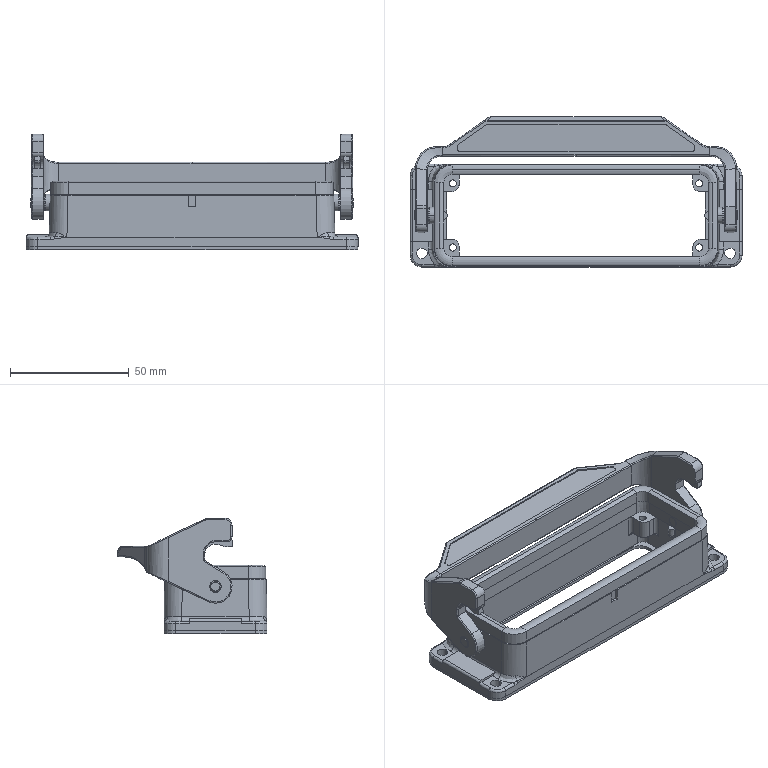Part | STEP file | 2 solids | 536 faces | box 140.01 x 63.21 x 48.7 mm | volume 56468 mm3 | plane 226 | cylinder 185 | spline 88 | torus 20 | cone 14 | sphere 3 | commonest cylinder face diameters 2 x37 1 x36 3 x19 10 x18 4 x12 7 x12